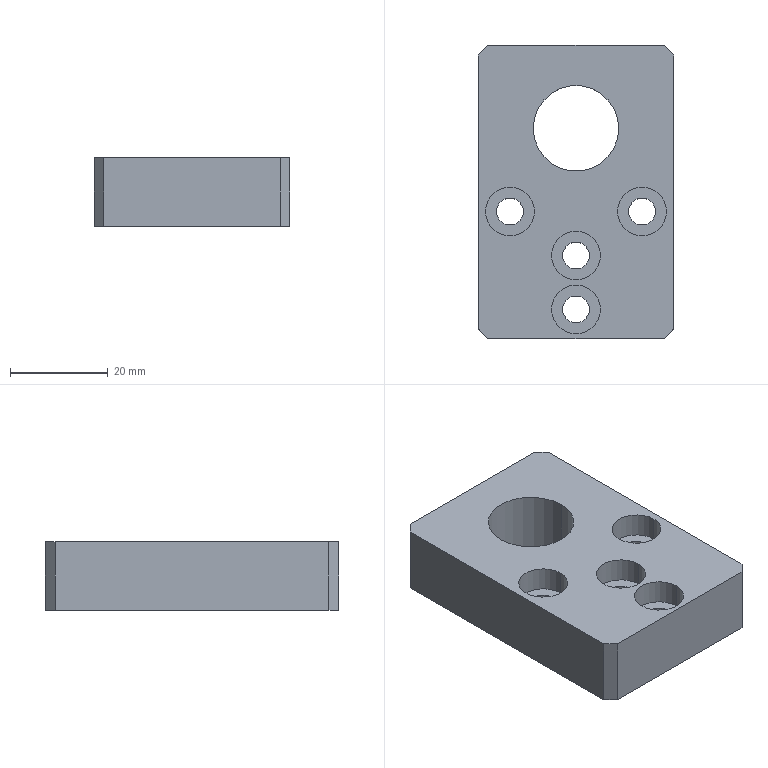Part | STEP file | adjusting nut 4 | 1 solid | 32 faces | box 40 x 60 x 14 mm | volume 27695 mm3 | cylinder 18 | plane 14 | commonest cylinder face diameters 5.5 x8 10 x8 17.5 x2